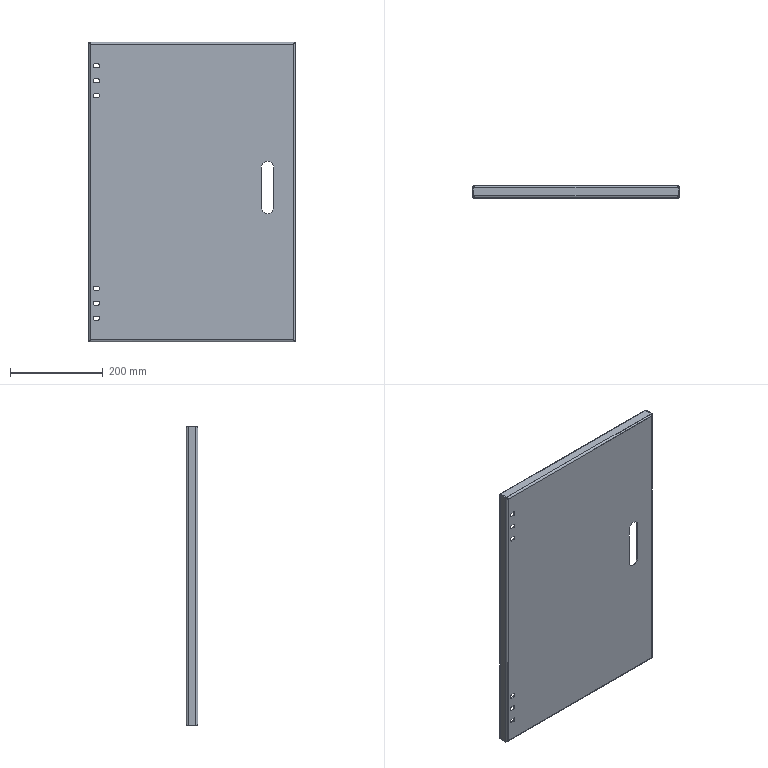Part | SolidWorks | features CornerFeat 4, ICE 3, EdgeFlange 2, Fillet 1, FlatPattern 1, SMBaseFlange 1, SheetMetal 1 | 1 solid | 120 faces | box 445 x 25 x 644 mm | volume 745118 mm3 | plane 60 | cylinder 44 | spline 16 | commonest cylinder face diameters 9 x18 4 x8 8 x8 6 x4 10 x4 26.5 x2